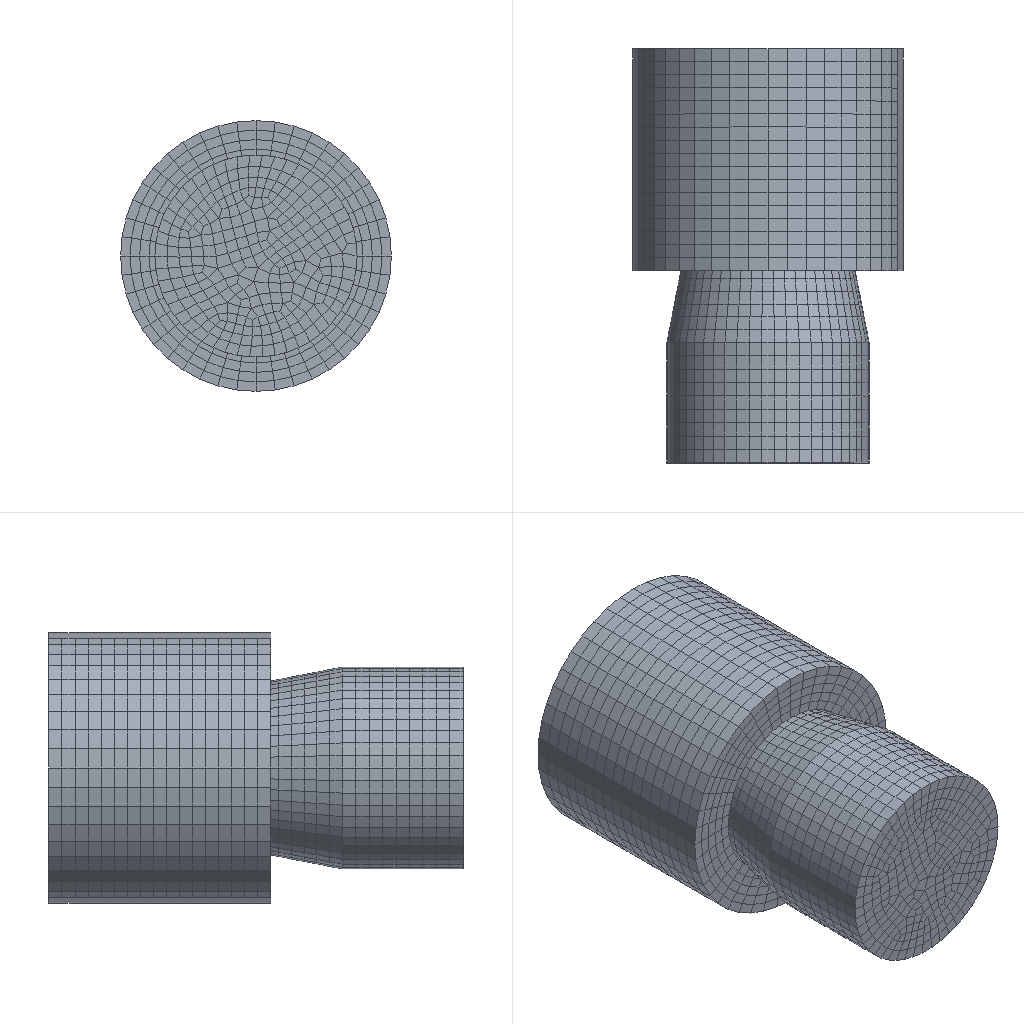Simulation study | abaqus
Set-up summary:
category,name,step,type,value,unit,region
solver,abaqus
solver,version,,,Abaqus/Explicit 2020
units,not stated in the deck,,not stated
analysis,deck,,dynamic temperature-displacement,dynamic temperature-displacement
load_step,Step-1,Step-1,dynamic temperature-displacement
load_step,requested,,,1
mesh,nodes,,,10912
mesh,elements,,,9098
element_type,C3D8RT,,solid,9098
load,load commands in deck,,count,2
bc,support commands in deck,,count,11
material,MATERIAL-1,,in results
material,MATERIAL-2,,in results
check,setup vs results,,match,"per instance, exact: element labels, types and connectivity; labels of the nodes the elements use; coordinates of those nodes at SINGLE_PRECISION in 2 of 2 instance(s)"
Abaqus input file, long lists of numbers shortened:
*Heading
** Job name: Job-1 Model name: Model-1
** Generated by: Abaqus/CAE 2020
*Preprint, echo=NO, model=NO, history=NO, contact=NO
**
** PARTS
**
*Part, name=TC18
*Node
      1,   30.026,         -72.,   7.709
      2,   27.166,         -72.,   14.934
** (6158 more lines like these left out)
*Element, type=C3D8RT
   1,  339,  373,  363,  312,   31,   65,   55,    4
   2,  568,  570,  431,  415,  260,  262,  123,  107
** (5356 more lines like these left out)
*Nset, nset=Set-1, generate
    1,  6160,     1
*Elset, elset=Set-1, generate
    1,  5358,     1
** Section: load
*Solid Section, elset=Set-1, material=Material-2
,
*End Part
**
*Part, name=Ti60
*Node
      1,         21.5,          68.,           0.
      2,         21.5,          28.,           0.
** (4750 more lines like these left out)
*Element, type=C3D8RT
  1,    1,   21,  377,   59,   89,  565, 2193,  658
  2,   21,   22,  378,  377,  565,  566, 2194, 2193
** (3738 more lines like these left out)
*Nset, nset=Set-2, generate
    1,  4752,     1
*Elset, elset=Set-2, generate
    1,  3740,     1
** Section: xuanzhuan
*Solid Section, elset=Set-2, material=Material-1
,
*End Part
**
**
** ASSEMBLY
**
*Assembly, name=Assembly
**
*Instance, name=TC18-1, part=TC18
          0.,          13.,           0.
*End Instance
**
*Instance, name=Ti60-1, part=Ti60
*End Instance
**
*Node
      1, -3.19720294e-15,          34.,           0.
*Node
      2,           0.,         -59., 1.89820253e-15
*Nset, nset=Set-2
 1,
*Nset, nset=Set-4
 2,
*Nset, nset=Set-5
 2,
*Nset, nset=m_Set-1
 1,
*Nset, nset=m_Set-3
 2,
*Elset, elset=_m_Surf-1_S1, internal, instance=TC18-1, generate
 5077,  5358,     1
*Elset, elset=_m_Surf-1_S6, internal, instance=TC18-1
    1,    6,   12,   16,   18,   23,   29,   30,   37,   40,   50,  283,  288,  294,  298,  300
  305,  311,  312,  319,  322,  332,  565,  570,  576,  580,  582,  587,  593,  594,  601,  604
** (12 more lines like these left out)
*Elset, elset=_m_Surf-1_S4, internal, instance=TC18-1
    3,    4,    8,   10,   11,   13,   14,   15,   17,   25,   28,   31,   32,   34,   35,   39
   43,   44,   45,   48,   49,   51,   52,   54,   55,   56,   58,   60,   63,   70,   71,   74
** (45 more lines like these left out)
*Surface, type=ELEMENT, name=m_Surf-1
_m_Surf-1_S1, S1
_m_Surf-1_S6, S6
_m_Surf-1_S4, S4
*Elset, elset=_s_Surf-3_S5, internal, instance=Ti60-1
   69,   70,   71,   72,   73,   74,   75,   76,   77,   78,   79,   80,   81,   82,   83,   84
   85,  154,  155,  156,  157,  158,  159,  160,  161,  162,  163,  164,  165,  166,  167,  168
** (45 more lines like these left out)
*Surface, type=ELEMENT, name=s_Surf-3
_s_Surf-3_S5, S5
*Elset, elset=_s_Surf-4_S2, internal, instance=TC18-1, generate
   1,  282,    1
*Surface, type=ELEMENT, name=s_Surf-4
_s_Surf-4_S2, S2
*Elset, elset=_s_Surf-5_S3, internal, instance=Ti60-1
    1,    2,    3,    4,    5,    6,    7,    8,    9,   10,   11,   12,   13,   14,   15,   16
   17,   86,   87,   88,   89,   90,   91,   92,   93,   94,   95,   96,   97,   98,   99,  100
** (45 more lines like these left out)
*Surface, type=ELEMENT, name=s_Surf-5
_s_Surf-5_S3, S3
** Constraint: Constraint-1
*Coupling, constraint name=Constraint-1, ref node=m_Set-1, surface=s_Surf-3
*Kinematic
** Constraint: Constraint-2
*Coupling, constraint name=Constraint-2, ref node=m_Set-3, surface=s_Surf-4
*Kinematic
*End Assembly
**
** MATERIALS
**
*Material, name=Material-1
*Conductivity
  7.5, 20.
  8.7,200.
 11.8,500.
*Density
 4.4e-09,
*Elastic
108000., 0.33
*Expansion
 9.1e-06, 20.
 9.2e-06,250.
 9.7e-06,500.
*Plastic, hardening=JOHNSON COOK
860., 683., 0.47,   1.,1650.,  25.
*Rate Dependent, type=JOHNSON COOK
 0.035,1.
*Specific Heat
 5.263e+08,
*Material, name=Material-2
*Conductivity
 12.5, 20.
 15.7,200.
 17.8,500.
*Density
 4.4e-09,
*Elastic
113000., 0.33
*Expansion
 9.04e-06, 20.
 9.14e-06,250.
 9.63e-06,500.
*Plastic, hardening=JOHNSON COOK
860., 683., 0.47,   1.,1650.,  25.
*Rate Dependent, type=JOHNSON COOK
 0.035,1.
*Specific Heat
 5.463e+08,
**
** INTERACTION PROPERTIES
**
*Surface Interaction, name=IntProp-1
*Friction
 0.15,
*Surface Behavior, pressure-overclosure=HARD
*Gap Conductance
 0.1,    0.
  0., 0.001
** ----------------------------------------------------------------
**
** STEP: Step-1
**
*Step, name=Step-1, nlgeom=YES
*Dynamic Temperature-displacement, Explicit
, 0.1
*Bulk Viscosity
0.06, 1.2
** Mass Scaling: Semi-Automatic
**               Whole Model
*Fixed Mass Scaling, factor=5000.
**
** BOUNDARY CONDITIONS
**
** Name: [REDACTED] : Displacement/rotation angle
*Boundary
Set-4, 1, 1
Set-4, 3, 3
Set-4, 4, 4
Set-4, 5, 5
Set-4, 6, 6
** Name: [REDACTED] : Velocity/Angular velocity
*Boundary, type=VELOCITY
Set-2, 1, 1
Set-2, 2, 2
Set-2, 3, 3
Set-2, 4, 4
Set-2, 5, 5, 100.
Set-2, 6, 6
**
** LOADS
**
** Name: Load-1   Type: Concentrated force
*Cload
Set-5, 2, 500000.
**
** INTERACTIONS
**
** Interaction: Int-1
*Contact Pair, interaction=IntProp-1, mechanical constraint=KINEMATIC, cpset=Int-1
m_Surf-1, s_Surf-5
**
** OUTPUT REQUESTS
**
*Restart, write, number interval=1, time marks=NO
**
** FIELD OUTPUT: F-Output-1
**
*Output, field, number interval=50
*Node Output
A, CF, NT, RF, RFL, RM, RT, U
V
*Element Output, directions=YES
E, EVF, HFL, LE, MISES, MISESMAX, MISESONLY, PE, PEEQ, PEEQMAX, PEEQT, PEEQVAVG, PEMAG, PEQC, PEVAVG, S
SSAVG, SVAVG, TEMP, YIELDPOT
*Contact Output
CDISP, CSTRESS
**
** HISTORY OUTPUT: H-Output-1
**
*Output, history, variable=PRESELECT
*End Step
Results summary:
result,step,Step-1,completed,increments=5330 time=0.1/0.1
result,analysis,,,"dynamic temperature-displacement, explict"
result,last_loadstep,,,1
result,primary field,,,"U, NT11"
result,reaction total,,FX,26899.739,model units
result,reaction total,,FY,-500204.625,model units
result,reaction total,,FZ,-139231.377,model units